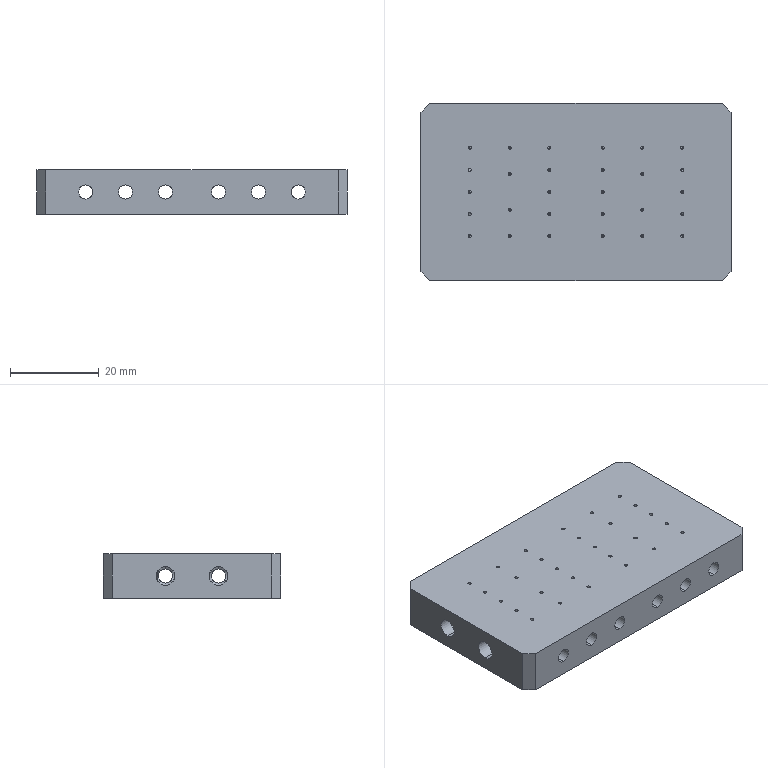Part | SolidWorks | features HoleWzd 8, LPattern 2, Chamfer 1, Extrusion 1 | 1 solid | 196 faces | box 70 x 40 x 10 mm | volume 24196 mm3 | cylinder 146 | cone 40 | plane 10 | commonest cylinder face diameters 3.2 x58 0.7 x56 4.2 x20 2.5 x12